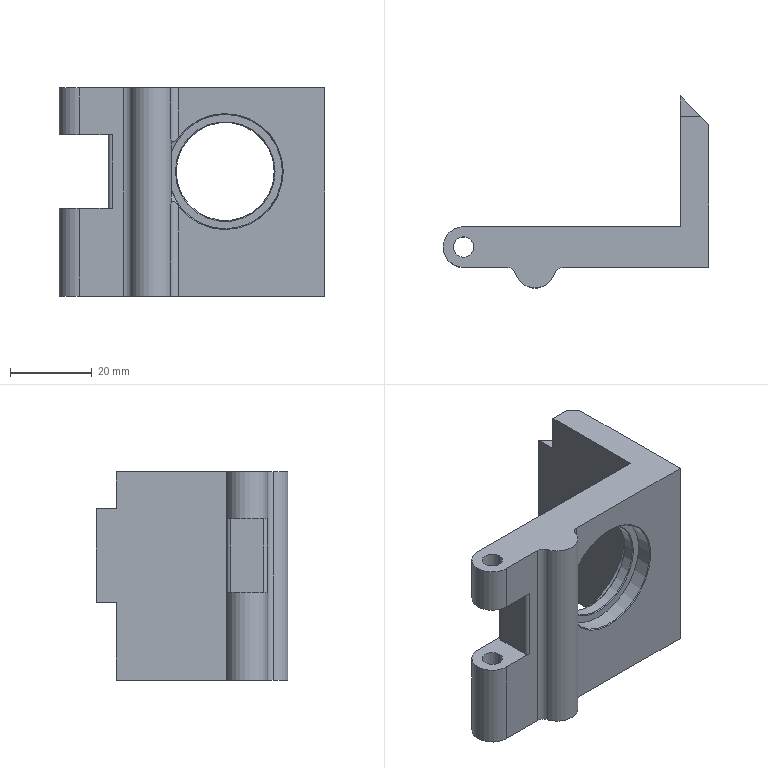Part | Creo | features CURVE 9, CUT 5, PROTRUSION 4, DATUM PLANE 3, ROUND 3, CHAMFER 2, COORDINATE SYSTEM 1 | 1 solid | 42 faces | box 65 x 47 x 51 mm | volume 35916 mm3 | cylinder 18 | plane 17 | cone 7 | commonest cylinder face diameters 5 x4 4 x3 10 x3 2 x2 24 x2 28 x2
STEP:
#1=CARTESIAN_POINT('',(0.,0.,0.));
#2=DIRECTION('',(0.,0.,1.));
#3=DIRECTION('',(1.,0.,0.));
#4=AXIS2_PLACEMENT_3D('',#1,#2,#3);
#5=CARTESIAN_POINT('',(28.,37.,20.5));
#6=VERTEX_POINT('',#5);
#7=CARTESIAN_POINT('',(33.,37.,20.5));
#8=VERTEX_POINT('',#7);
#9=CARTESIAN_POINT('',(28.,37.,20.5));
#10=DIRECTION('',(1.,0.,0.));
#11=VECTOR('',#10,5.);
#12=LINE('',#9,#11);
#13=EDGE_CURVE('',#6,#8,#12,.T.);
#14=ORIENTED_EDGE('',*,*,#13,.T.);
#15=CARTESIAN_POINT('',(35.,35.,20.5));
#16=VERTEX_POINT('',#15);
#17=CARTESIAN_POINT('',(35.,35.,20.5));
#18=DIRECTION('',(-0.7071,0.7071,0.));
#19=VECTOR('',#18,2.828);
#20=LINE('',#17,#19);
#21=EDGE_CURVE('',#16,#8,#20,.T.);
#22=ORIENTED_EDGE('',*,*,#21,.F.);
#23=CARTESIAN_POINT('',(35.,0.,20.5));
#24=VERTEX_POINT('',#23);
#25=CARTESIAN_POINT('',(35.,35.,20.5));
#26=DIRECTION('',(0.,-1.,0.));
#27=VECTOR('',#26,35.);
#28=LINE('',#25,#27);
#29=EDGE_CURVE('',#16,#24,#28,.T.);
#30=ORIENTED_EDGE('',*,*,#29,.T.);
#31=CARTESIAN_POINT('',(-0.7918,0.,20.5));
#32=VERTEX_POINT('',#31);
#33=CARTESIAN_POINT('',(35.,0.,20.5));
#34=DIRECTION('',(-1.,0.,0.));
#35=VECTOR('',#34,35.792);
#36=LINE('',#33,#35);
#37=EDGE_CURVE('',#24,#32,#36,.T.);
#38=ORIENTED_EDGE('',*,*,#37,.T.);
#39=CARTESIAN_POINT('',(-2.708,-1.429,20.5));
#40=VERTEX_POINT('',#39);
#41=CARTESIAN_POINT('',(-0.7918,-2.,20.5));
#42=DIRECTION('',(0.,0.,-1.));
#43=DIRECTION('',(-0.9583,0.2857,0.));
#44=AXIS2_PLACEMENT_3D('',#41,#42,#43);
#45=CIRCLE('',#44,2.);
#46=EDGE_CURVE('',#40,#32,#45,.T.);
#47=ORIENTED_EDGE('',*,*,#46,.F.);
#48=CARTESIAN_POINT('',(-12.292,-1.429,20.5));
#49=VERTEX_POINT('',#48);
#50=CARTESIAN_POINT('',(-7.5,0.,20.5));
#51=DIRECTION('',(0.,0.,1.));
#52=DIRECTION('',(-0.9583,-0.2857,0.));
#53=AXIS2_PLACEMENT_3D('',#50,#51,#52);
#54=CIRCLE('',#53,5.);
#55=EDGE_CURVE('',#49,#40,#54,.T.);
#56=ORIENTED_EDGE('',*,*,#55,.F.);
#57=CARTESIAN_POINT('',(-14.208,0.,20.5));
#58=VERTEX_POINT('',#57);
#59=CARTESIAN_POINT('',(-14.208,-2.,20.5));
#60=DIRECTION('',(0.,0.,-1.));
#61=DIRECTION('',(0.,1.,0.));
#62=AXIS2_PLACEMENT_3D('',#59,#60,#61);
#63=CIRCLE('',#62,2.);
#64=EDGE_CURVE('',#58,#49,#63,.T.);
#65=ORIENTED_EDGE('',*,*,#64,.F.);
#66=CARTESIAN_POINT('',(-25.,0.,20.5));
#67=VERTEX_POINT('',#66);
#68=CARTESIAN_POINT('',(-25.,0.,20.5));
#69=DIRECTION('',(1.,0.,0.));
#70=VECTOR('',#69,10.792);
#71=LINE('',#68,#70);
#72=EDGE_CURVE('',#67,#58,#71,.T.);
#73=ORIENTED_EDGE('',*,*,#72,.F.);
#74=CARTESIAN_POINT('',(-25.,10.,20.5));
#75=VERTEX_POINT('',#74);
#76=CARTESIAN_POINT('',(-25.,5.,20.5));
#77=DIRECTION('',(0.,0.,-1.));
#78=DIRECTION('',(0.,-1.,0.));
#79=AXIS2_PLACEMENT_3D('',#76,#77,#78);
#80=CIRCLE('',#79,5.);
#81=EDGE_CURVE('',#67,#75,#80,.T.);
#82=ORIENTED_EDGE('',*,*,#81,.T.);
#83=CARTESIAN_POINT('',(28.,10.,20.5));
#84=VERTEX_POINT('',#83);
#85=CARTESIAN_POINT('',(28.,10.,20.5));
#86=DIRECTION('',(-1.,0.,0.));
#87=VECTOR('',#86,53.);
#88=LINE('',#85,#87);
#89=EDGE_CURVE('',#84,#75,#88,.T.);
#90=ORIENTED_EDGE('',*,*,#89,.F.);
#91=CARTESIAN_POINT('',(28.,37.,20.5));
#92=DIRECTION('',(0.,-1.,0.));
#93=VECTOR('',#92,27.);
#94=LINE('',#91,#93);
#95=EDGE_CURVE('',#6,#84,#94,.T.);
#96=ORIENTED_EDGE('',*,*,#95,.F.);
#97=EDGE_LOOP('',(#14,#22,#30,#38,#47,#56,#65,#73,#82,#90,#96));
#98=FACE_OUTER_BOUND('',#97,.F.);
#99=CARTESIAN_POINT('',(-22.5,5.,20.5));
#100=VERTEX_POINT('',#99);
#101=CARTESIAN_POINT('',(-27.5,5.,20.5));
#102=VERTEX_POINT('',#101);
#103=CARTESIAN_POINT('',(-25.,5.,20.5));
#104=DIRECTION('',(0.,0.,-1.));
#105=DIRECTION('',(1.,0.,0.));
#106=AXIS2_PLACEMENT_3D('',#103,#104,#105);
#107=CIRCLE('',#106,2.5);
#108=EDGE_CURVE('',#100,#102,#107,.T.);
#109=ORIENTED_EDGE('',*,*,#108,.F.);
#110=CARTESIAN_POINT('',(-25.,5.,20.5));
#111=DIRECTION('',(0.,0.,-1.));
#112=DIRECTION('',(-1.,0.,0.));
#113=AXIS2_PLACEMENT_3D('',#110,#111,#112);
#114=CIRCLE('',#113,2.5);
#115=EDGE_CURVE('',#102,#100,#114,.T.);
#116=ORIENTED_EDGE('',*,*,#115,.F.);
#117=EDGE_LOOP('',(#109,#116));
#118=FACE_BOUND('',#117,.F.);
#119=CARTESIAN_POINT('',(0.,0.,20.5));
#120=DIRECTION('',(0.,0.,1.));
#121=DIRECTION('',(1.,0.,0.));
#122=AXIS2_PLACEMENT_3D('',#119,#120,#121);
#123=PLANE('',#122);
#124=ADVANCED_FACE('',(#98,#118),#123,.T.);
#125=CARTESIAN_POINT('',(-27.5,5.,9.));
#126=VERTEX_POINT('',#125);
#127=CARTESIAN_POINT('',(-22.5,5.,9.));
#128=VERTEX_POINT('',#127);
#129=CARTESIAN_POINT('',(-25.,5.,9.));
#130=DIRECTION('',(0.,0.,1.));
#131=DIRECTION('',(-1.,0.,0.));
#132=AXIS2_PLACEMENT_3D('',#129,#130,#131);
#133=CIRCLE('',#132,2.5);
#134=EDGE_CURVE('',#126,#128,#133,.T.);
#135=ORIENTED_EDGE('',*,*,#134,.T.);
#136=CARTESIAN_POINT('',(-22.5,5.,9.));
#137=DIRECTION('',(0.,0.,1.));
#138=VECTOR('',#137,11.5);
#139=LINE('',#136,#138);
#140=EDGE_CURVE('',#128,#100,#139,.T.);
#141=ORIENTED_EDGE('',*,*,#140,.T.);
#142=ORIENTED_EDGE('',*,*,#108,.T.);
#143=CARTESIAN_POINT('',(-27.5,5.,9.));
#144=DIRECTION('',(0.,0.,1.));
#145=VECTOR('',#144,11.5);
#146=LINE('',#143,#145);
#147=EDGE_CURVE('',#126,#102,#146,.T.);
#148=ORIENTED_EDGE('',*,*,#147,.F.);
#149=EDGE_LOOP('',(#135,#141,#142,#148));
#150=FACE_OUTER_BOUND('',#149,.F.);
#151=CARTESIAN_POINT('',(-25.,5.,-20.5));
#152=DIRECTION('',(0.,0.,1.));
#153=DIRECTION('',(1.,0.,0.));
#154=AXIS2_PLACEMENT_3D('',#151,#152,#153);
#155=CYLINDRICAL_SURFACE('',#154,2.5);
#156=ADVANCED_FACE('',(#150),#155,.F.);
#157=CARTESIAN_POINT('',(-27.5,5.,-9.));
#158=VERTEX_POINT('',#157);
#159=CARTESIAN_POINT('',(-27.5,5.,-30.5));
#160=VERTEX_POINT('',#159);
#161=CARTESIAN_POINT('',(-27.5,5.,-9.));
#162=DIRECTION('',(0.,0.,-1.));
#163=VECTOR('',#162,21.5);
#164=LINE('',#161,#163);
#165=EDGE_CURVE('',#158,#160,#164,.T.);
#166=ORIENTED_EDGE('',*,*,#165,.T.);
#167=CARTESIAN_POINT('',(-22.5,5.,-30.5));
#168=VERTEX_POINT('',#167);
#169=CARTESIAN_POINT('',(-25.,5.,-30.5));
#170=DIRECTION('',(0.,0.,1.));
#171=DIRECTION('',(-1.,0.,0.));
#172=AXIS2_PLACEMENT_3D('',#169,#170,#171);
#173=CIRCLE('',#172,2.5);
#174=EDGE_CURVE('',#160,#168,#173,.T.);
#175=ORIENTED_EDGE('',*,*,#174,.T.);
#176=CARTESIAN_POINT('',(-22.5,5.,-9.));
#177=VERTEX_POINT('',#176);
#178=CARTESIAN_POINT('',(-22.5,5.,-30.5));
#179=DIRECTION('',(0.,0.,1.));
#180=VECTOR('',#179,21.5);
#181=LINE('',#178,#180);
#182=EDGE_CURVE('',#168,#177,#181,.T.);
#183=ORIENTED_EDGE('',*,*,#182,.T.);
#184=CARTESIAN_POINT('',(-25.,5.,-9.));
#185=DIRECTION('',(0.,0.,1.));
#186=DIRECTION('',(-1.,0.,0.));
#187=AXIS2_PLACEMENT_3D('',#184,#185,#186);
#188=CIRCLE('',#187,2.5);
#189=EDGE_CURVE('',#158,#177,#188,.T.);
#190=ORIENTED_EDGE('',*,*,#189,.F.);
#191=EDGE_LOOP('',(#166,#175,#183,#190));
#192=FACE_OUTER_BOUND('',#191,.F.);
#193=CARTESIAN_POINT('',(-25.,5.,-20.5));
#194=DIRECTION('',(0.,0.,1.));
#195=DIRECTION('',(1.,0.,0.));
#196=AXIS2_PLACEMENT_3D('',#193,#194,#195);
#197=CYLINDRICAL_SURFACE('',#196,2.5);
#198=ADVANCED_FACE('',(#192),#197,.F.);
#199=CARTESIAN_POINT('',(-25.,0.,9.));
#200=VERTEX_POINT('',#199);
#201=CARTESIAN_POINT('',(-17.,0.,9.));
#202=VERTEX_POINT('',#201);
#203=CARTESIAN_POINT('',(-25.,0.,9.));
#204=DIRECTION('',(1.,0.,0.));
#205=VECTOR('',#204,8.);
#206=LINE('',#203,#205);
#207=EDGE_CURVE('',#200,#202,#206,.T.);
#208=ORIENTED_EDGE('',*,*,#207,.T.);
#209=CARTESIAN_POINT('',(-18.,1.,9.));
#210=VERTEX_POINT('',#209);
#211=CARTESIAN_POINT('',(-17.,1.,9.));
#212=DIRECTION('',(0.,0.,1.));
#213=DIRECTION('',(-1.,0.,0.));
#214=AXIS2_PLACEMENT_3D('',#211,#212,#213);
#215=CIRCLE('',#214,1.);
#216=EDGE_CURVE('',#210,#202,#215,.T.);
#217=ORIENTED_EDGE('',*,*,#216,.F.);
#218=CARTESIAN_POINT('',(-18.,9.,9.));
#219=VERTEX_POINT('',#218);
#220=CARTESIAN_POINT('',(-18.,9.,9.));
#221=DIRECTION('',(0.,-1.,0.));
#222=VECTOR('',#221,8.);
#223=LINE('',#220,#222);
#224=EDGE_CURVE('',#219,#210,#223,.T.);
#225=ORIENTED_EDGE('',*,*,#224,.F.);
#226=CARTESIAN_POINT('',(-17.,10.,9.));
#227=VERTEX_POINT('',#226);
#228=CARTESIAN_POINT('',(-17.,9.,9.));
#229=DIRECTION('',(0.,0.,1.));
#230=DIRECTION('',(0.,1.,0.));
#231=AXIS2_PLACEMENT_3D('',#228,#229,#230);
#232=CIRCLE('',#231,1.);
#233=EDGE_CURVE('',#227,#219,#232,.T.);
#234=ORIENTED_EDGE('',*,*,#233,.F.);
#235=CARTESIAN_POINT('',(-25.,10.,9.));
#236=VERTEX_POINT('',#235);
#237=CARTESIAN_POINT('',(-17.,10.,9.));
#238=DIRECTION('',(-1.,0.,0.));
#239=VECTOR('',#238,8.);
#240=LINE('',#237,#239);
#241=EDGE_CURVE('',#227,#236,#240,.T.);
#242=ORIENTED_EDGE('',*,*,#241,.T.);
#243=CARTESIAN_POINT('',(-25.,5.,9.));
#244=DIRECTION('',(0.,0.,1.));
#245=DIRECTION('',(0.,1.,0.));
#246=AXIS2_PLACEMENT_3D('',#243,#244,#245);
#247=CIRCLE('',#246,5.);
#248=EDGE_CURVE('',#236,#200,#247,.T.);
#249=ORIENTED_EDGE('',*,*,#248,.T.);
#250=EDGE_LOOP('',(#208,#217,#225,#234,#242,#249));
#251=FACE_OUTER_BOUND('',#250,.F.);
#252=ORIENTED_EDGE('',*,*,#134,.F.);
#253=CARTESIAN_POINT('',(-25.,5.,9.));
#254=DIRECTION('',(0.,0.,1.));
#255=DIRECTION('',(1.,0.,0.));
#256=AXIS2_PLACEMENT_3D('',#253,#254,#255);
#257=CIRCLE('',#256,2.5);
#258=EDGE_CURVE('',#128,#126,#257,.T.);
#259=ORIENTED_EDGE('',*,*,#258,.F.);
#260=EDGE_LOOP('',(#252,#259));
#261=FACE_BOUND('',#260,.F.);
#262=CARTESIAN_POINT('',(-30.,10.,9.));
#263=DIRECTION('',(0.,0.,1.));
#264=DIRECTION('',(1.,0.,0.));
#265=AXIS2_PLACEMENT_3D('',#262,#263,#264);
#266=PLANE('',#265);
#267=ADVANCED_FACE('',(#251,#261),#266,.F.);
#268=ORIENTED_EDGE('',*,*,#258,.T.);
#269=ORIENTED_EDGE('',*,*,#147,.T.);
#270=ORIENTED_EDGE('',*,*,#115,.T.);
#271=ORIENTED_EDGE('',*,*,#140,.F.);
#272=EDGE_LOOP('',(#268,#269,#270,#271));
#273=FACE_OUTER_BOUND('',#272,.F.);
#274=CARTESIAN_POINT('',(-25.,5.,-20.5));
#275=DIRECTION('',(0.,0.,1.));
#276=DIRECTION('',(1.,0.,0.));
#277=AXIS2_PLACEMENT_3D('',#274,#275,#276);
#278=CYLINDRICAL_SURFACE('',#277,2.5);
#279=ADVANCED_FACE('',(#273),#278,.F.);
#280=ORIENTED_EDGE('',*,*,#182,.F.);
#281=CARTESIAN_POINT('',(-25.,5.,-30.5));
#282=DIRECTION('',(0.,0.,1.));
#283=DIRECTION('',(1.,0.,0.));
#284=AXIS2_PLACEMENT_3D('',#281,#282,#283);
#285=CIRCLE('',#284,2.5);
#286=EDGE_CURVE('',#168,#160,#285,.T.);
#287=ORIENTED_EDGE('',*,*,#286,.T.);
#288=ORIENTED_EDGE('',*,*,#165,.F.);
#289=CARTESIAN_POINT('',(-25.,5.,-9.));
#290=DIRECTION('',(0.,0.,1.));
#291=DIRECTION('',(1.,0.,0.));
#292=AXIS2_PLACEMENT_3D('',#289,#290,#291);
#293=CIRCLE('',#292,2.5);
#294=EDGE_CURVE('',#177,#158,#293,.T.);
#295=ORIENTED_EDGE('',*,*,#294,.F.);
#296=EDGE_LOOP('',(#280,#287,#288,#295));
#297=FACE_OUTER_BOUND('',#296,.F.);
#298=CARTESIAN_POINT('',(-25.,5.,-20.5));
#299=DIRECTION('',(0.,0.,1.));
#300=DIRECTION('',(1.,0.,0.));
#301=AXIS2_PLACEMENT_3D('',#298,#299,#300);
#302=CYLINDRICAL_SURFACE('',#301,2.5);
#303=ADVANCED_FACE('',(#297),#302,.F.);
#304=CARTESIAN_POINT('',(33.,37.,-30.5));
#305=VERTEX_POINT('',#304);
#306=CARTESIAN_POINT('',(28.,37.,-30.5));
#307=VERTEX_POINT('',#306);
#308=CARTESIAN_POINT('',(33.,37.,-30.5));
#309=DIRECTION('',(-1.,0.,0.));
#310=VECTOR('',#309,5.);
#311=LINE('',#308,#310);
#312=EDGE_CURVE('',#305,#307,#311,.T.);
#313=ORIENTED_EDGE('',*,*,#312,.T.);
#314=CARTESIAN_POINT('',(28.,10.,-30.5));
#315=VERTEX_POINT('',#314);
#316=CARTESIAN_POINT('',(28.,10.,-30.5));
#317=DIRECTION('',(0.,1.,0.));
#318=VECTOR('',#317,27.);
#319=LINE('',#316,#318);
#320=EDGE_CURVE('',#315,#307,#319,.T.);
#321=ORIENTED_EDGE('',*,*,#320,.F.);
#322=CARTESIAN_POINT('',(-25.,10.,-30.5));
#323=VERTEX_POINT('',#322);
#324=CARTESIAN_POINT('',(-25.,10.,-30.5));
#325=DIRECTION('',(1.,0.,0.));
#326=VECTOR('',#325,53.);
#327=LINE('',#324,#326);
#328=EDGE_CURVE('',#323,#315,#327,.T.);
#329=ORIENTED_EDGE('',*,*,#328,.F.);
#330=CARTESIAN_POINT('',(-25.,0.,-30.5));
#331=VERTEX_POINT('',#330);
#332=CARTESIAN_POINT('',(-25.,5.,-30.5));
#333=DIRECTION('',(0.,0.,-1.));
#334=DIRECTION('',(0.,-1.,0.));
#335=AXIS2_PLACEMENT_3D('',#332,#333,#334);
#336=CIRCLE('',#335,5.);
#337=EDGE_CURVE('',#331,#323,#336,.T.);
#338=ORIENTED_EDGE('',*,*,#337,.F.);
#339=CARTESIAN_POINT('',(-14.208,0.,-30.5));
#340=VERTEX_POINT('',#339);
#341=CARTESIAN_POINT('',(-14.208,0.,-30.5));
#342=DIRECTION('',(-1.,0.,0.));
#343=VECTOR('',#342,10.792);
#344=LINE('',#341,#343);
#345=EDGE_CURVE('',#340,#331,#344,.T.);
#346=ORIENTED_EDGE('',*,*,#345,.F.);
#347=CARTESIAN_POINT('',(-12.292,-1.429,-30.5));
#348=VERTEX_POINT('',#347);
#349=CARTESIAN_POINT('',(-14.208,-2.,-30.5));
#350=DIRECTION('',(0.,0.,1.));
#351=DIRECTION('',(0.9583,0.2857,0.));
#352=AXIS2_PLACEMENT_3D('',#349,#350,#351);
#353=CIRCLE('',#352,2.);
#354=EDGE_CURVE('',#348,#340,#353,.T.);
#355=ORIENTED_EDGE('',*,*,#354,.F.);
#356=CARTESIAN_POINT('',(-2.708,-1.429,-30.5));
#357=VERTEX_POINT('',#356);
#358=CARTESIAN_POINT('',(-7.5,0.,-30.5));
#359=DIRECTION('',(0.,0.,-1.));
#360=DIRECTION('',(0.9583,-0.2857,0.));
#361=AXIS2_PLACEMENT_3D('',#358,#359,#360);
#362=CIRCLE('',#361,5.);
#363=EDGE_CURVE('',#357,#348,#362,.T.);
#364=ORIENTED_EDGE('',*,*,#363,.F.);
#365=CARTESIAN_POINT('',(-0.7918,0.,-30.5));
#366=VERTEX_POINT('',#365);
#367=CARTESIAN_POINT('',(-0.7918,-2.,-30.5));
#368=DIRECTION('',(0.,0.,1.));
#369=DIRECTION('',(0.,1.,0.));
#370=AXIS2_PLACEMENT_3D('',#367,#368,#369);
#371=CIRCLE('',#370,2.);
#372=EDGE_CURVE('',#366,#357,#371,.T.);
#373=ORIENTED_EDGE('',*,*,#372,.F.);
#374=CARTESIAN_POINT('',(35.,0.,-30.5));
#375=VERTEX_POINT('',#374);
#376=CARTESIAN_POINT('',(-0.7918,0.,-30.5));
#377=DIRECTION('',(1.,0.,0.));
#378=VECTOR('',#377,35.792);
#379=LINE('',#376,#378);
#380=EDGE_CURVE('',#366,#375,#379,.T.);
#381=ORIENTED_EDGE('',*,*,#380,.T.);
#382=CARTESIAN_POINT('',(35.,35.,-30.5));
#383=VERTEX_POINT('',#382);
#384=CARTESIAN_POINT('',(35.,0.,-30.5));
#385=DIRECTION('',(0.,1.,0.));
#386=VECTOR('',#385,35.);
#387=LINE('',#384,#386);
#388=EDGE_CURVE('',#375,#383,#387,.T.);
#389=ORIENTED_EDGE('',*,*,#388,.T.);
#390=CARTESIAN_POINT('',(33.,37.,-30.5));
#391=DIRECTION('',(0.7071,-0.7071,0.));
#392=VECTOR('',#391,2.828);
#393=LINE('',#390,#392);
#394=EDGE_CURVE('',#305,#383,#393,.T.);
#395=ORIENTED_EDGE('',*,*,#394,.F.);
#396=EDGE_LOOP('',(#313,#321,#329,#338,#346,#355,#364,#373,#381,#389,#395));
#397=FACE_OUTER_BOUND('',#396,.F.);
#398=ORIENTED_EDGE('',*,*,#286,.F.);
#399=ORIENTED_EDGE('',*,*,#174,.F.);
#400=EDGE_LOOP('',(#398,#399));
#401=FACE_BOUND('',#400,.F.);
#402=CARTESIAN_POINT('',(0.,0.,-30.5));
#403=DIRECTION('',(0.,0.,-1.));
#404=DIRECTION('',(-1.,0.,0.));
#405=AXIS2_PLACEMENT_3D('',#402,#403,#404);
#406=PLANE('',#405);
#407=ADVANCED_FACE('',(#397,#401),#406,.T.);
#408=CARTESIAN_POINT('',(28.,37.,-11.5));
#409=VERTEX_POINT('',#408);
#410=CARTESIAN_POINT('',(28.,37.,-30.5));
#411=DIRECTION('',(0.,0.,1.));
#412=VECTOR('',#411,19.);
#413=LINE('',#410,#412);
#414=EDGE_CURVE('',#307,#409,#413,.T.);
#415=ORIENTED_EDGE('',*,*,#414,.F.);
#416=ORIENTED_EDGE('',*,*,#312,.F.);
#417=CARTESIAN_POINT('',(33.,37.,-11.5));
#418=VERTEX_POINT('',#417);
#419=CARTESIAN_POINT('',(33.,37.,-30.5));
#420=DIRECTION('',(0.,0.,1.));
#421=VECTOR('',#420,19.);
#422=LINE('',#419,#421);
#423=EDGE_CURVE('',#305,#418,#422,.T.);
#424=ORIENTED_EDGE('',*,*,#423,.T.);
#425=CARTESIAN_POINT('',(33.,37.,-11.5));
#426=DIRECTION('',(-1.,0.,0.));
#427=VECTOR('',#426,5.);
#428=LINE('',#425,#427);
#429=EDGE_CURVE('',#418,#409,#428,.T.);
#430=ORIENTED_EDGE('',*,*,#429,.T.);
#431=EDGE_LOOP('',(#415,#416,#424,#430));
#432=FACE_OUTER_BOUND('',#431,.F.);
#433=CARTESIAN_POINT('',(35.,37.,-11.5));
#434=DIRECTION('',(0.,-1.,0.));
#435=DIRECTION('',(0.,0.,-1.));
#436=AXIS2_PLACEMENT_3D('',#433,#434,#435);
#437=PLANE('',#436);
#438=ADVANCED_FACE('',(#432),#437,.F.);
#439=CARTESIAN_POINT('',(28.,42.,-11.5));
#440=VERTEX_POINT('',#439);
#441=CARTESIAN_POINT('',(28.,42.,-11.5));
#442=DIRECTION('',(0.,-1.,0.));
#443=VECTOR('',#442,5.);
#444=LINE('',#441,#443);
#445=EDGE_CURVE('',#440,#409,#444,.T.);
#446=ORIENTED_EDGE('',*,*,#445,.F.);
#447=CARTESIAN_POINT('',(28.,42.,11.5));
#448=VERTEX_POINT('',#447);
#449=CARTESIAN_POINT('',(28.,42.,-11.5));
#450=DIRECTION('',(0.,0.,1.));
#451=VECTOR('',#450,23.);
#452=LINE('',#449,#451);
#453=EDGE_CURVE('',#440,#448,#452,.T.);
#454=ORIENTED_EDGE('',*,*,#453,.T.);
#455=CARTESIAN_POINT('',(28.,37.,11.5));
#456=VERTEX_POINT('',#455);
#457=CARTESIAN_POINT('',(28.,42.,11.5));
#458=DIRECTION('',(0.,-1.,0.));
#459=VECTOR('',#458,5.);
#460=LINE('',#457,#459);
#461=EDGE_CURVE('',#448,#456,#460,.T.);
#462=ORIENTED_EDGE('',*,*,#461,.T.);
#463=CARTESIAN_POINT('',(28.,37.,20.5));
#464=DIRECTION('',(0.,0.,-1.));
#465=VECTOR('',#464,9.);
#466=LINE('',#463,#465);
#467=EDGE_CURVE('',#6,#456,#466,.T.);
#468=ORIENTED_EDGE('',*,*,#467,.F.);
#469=ORIENTED_EDGE('',*,*,#95,.T.);
#470=CARTESIAN_POINT('',(28.,10.,20.5));
#471=DIRECTION('',(0.,0.,-1.));
#472=VECTOR('',#471,51.);
#473=LINE('',#470,#472);
#474=EDGE_CURVE('',#84,#315,#473,.T.);
#475=ORIENTED_EDGE('',*,*,#474,.T.);
#476=ORIENTED_EDGE('',*,*,#320,.T.);
#477=ORIENTED_EDGE('',*,*,#414,.T.);
#478=EDGE_LOOP('',(#446,#454,#462,#468,#469,#475,#476,#477));
#479=FACE_OUTER_BOUND('',#478,.F.);
#480=CARTESIAN_POINT('',(28.,42.,-20.5));
#481=DIRECTION('',(-1.,0.,0.));
#482=DIRECTION('',(0.,-1.,0.));
#483=AXIS2_PLACEMENT_3D('',#480,#481,#482);
#484=PLANE('',#483);
#485=ADVANCED_FACE('',(#479),#484,.T.);
#486=ORIENTED_EDGE('',*,*,#445,.T.);
#487=ORIENTED_EDGE('',*,*,#429,.F.);
#488=CARTESIAN_POINT('',(28.,42.,-11.5));
#489=DIRECTION('',(0.7071,-0.7071,0.));
#490=VECTOR('',#489,7.071);
#491=LINE('',#488,#490);
#492=EDGE_CURVE('',#440,#418,#491,.T.);
#493=ORIENTED_EDGE('',*,*,#492,.F.);
#494=EDGE_LOOP('',(#486,#487,#493));
#495=FACE_OUTER_BOUND('',#494,.F.);
#496=CARTESIAN_POINT('',(35.,42.,-11.5));
#497=DIRECTION('',(0.,0.,1.));
#498=DIRECTION('',(0.,-1.,0.));
#499=AXIS2_PLACEMENT_3D('',#496,#497,#498);
#500=PLANE('',#499);
#501=ADVANCED_FACE('',(#495),#500,.F.);
#502=ORIENTED_EDGE('',*,*,#492,.T.);
#503=ORIENTED_EDGE('',*,*,#423,.F.);
#504=ORIENTED_EDGE('',*,*,#394,.T.);
#505=CARTESIAN_POINT('',(35.,35.,-30.5));
#506=DIRECTION('',(0.,0.,1.));
#507=VECTOR('',#506,51.);
#508=LINE('',#505,#507);
#509=EDGE_CURVE('',#383,#16,#508,.T.);
#510=ORIENTED_EDGE('',*,*,#509,.T.);
#511=ORIENTED_EDGE('',*,*,#21,.T.);
#512=CARTESIAN_POINT('',(33.,37.,11.5));
#513=VERTEX_POINT('',#512);
#514=CARTESIAN_POINT('',(33.,37.,20.5));
#515=DIRECTION('',(0.,0.,-1.));
#516=VECTOR('',#515,9.);
#517=LINE('',#514,#516);
#518=EDGE_CURVE('',#8,#513,#517,.T.);
#519=ORIENTED_EDGE('',*,*,#518,.T.);
#520=CARTESIAN_POINT('',(28.,42.,11.5));
#521=DIRECTION('',(0.7071,-0.7071,0.));
#522=VECTOR('',#521,7.071);
#523=LINE('',#520,#522);
#524=EDGE_CURVE('',#448,#513,#523,.T.);
#525=ORIENTED_EDGE('',*,*,#524,.F.);
#526=ORIENTED_EDGE('',*,*,#453,.F.);
#527=EDGE_LOOP('',(#502,#503,#504,#510,#511,#519,#525,#526));
#528=FACE_OUTER_BOUND('',#527,.F.);
#529=CARTESIAN_POINT('',(31.5,38.5,-5.));
#530=DIRECTION('',(0.7071,0.7071,0.));
#531=DIRECTION('',(-0.7071,0.7071,0.));
#532=AXIS2_PLACEMENT_3D('',#529,#530,#531);
#533=PLANE('',#532);
#534=ADVANCED_FACE('',(#528),#533,.T.);
#535=ORIENTED_EDGE('',*,*,#509,.F.);
#536=ORIENTED_EDGE('',*,*,#388,.F.);
#537=CARTESIAN_POINT('',(35.,0.,20.5));
#538=DIRECTION('',(0.,0.,-1.));
#539=VECTOR('',#538,51.);
#540=LINE('',#537,#539);
#541=EDGE_CURVE('',#24,#375,#540,.T.);
#542=ORIENTED_EDGE('',*,*,#541,.F.);
#543=ORIENTED_EDGE('',*,*,#29,.F.);
#544=EDGE_LOOP('',(#535,#536,#542,#543));
#545=FACE_OUTER_BOUND('',#544,.F.);
#546=CARTESIAN_POINT('',(35.,0.,20.5));
#547=DIRECTION('',(1.,0.,0.));
#548=DIRECTION('',(0.,0.,-1.));
#549=AXIS2_PLACEMENT_3D('',#546,#547,#548);
#550=PLANE('',#549);
#551=ADVANCED_FACE('',(#545),#550,.T.);
#552=CARTESIAN_POINT('',(-14.208,0.,-30.5));
#553=DIRECTION('',(0.,0.,1.));
#554=VECTOR('',#553,51.);
#555=LINE('',#552,#554);
#556=EDGE_CURVE('',#340,#58,#555,.T.);
#557=ORIENTED_EDGE('',*,*,#556,.F.);
#558=ORIENTED_EDGE('',*,*,#345,.T.);
#559=CARTESIAN_POINT('',(-25.,0.,-9.));
#560=VERTEX_POINT('',#559);
#561=CARTESIAN_POINT('',(-25.,0.,-30.5));
#562=DIRECTION('',(0.,0.,1.));
#563=VECTOR('',#562,21.5);
#564=LINE('',#561,#563);
#565=EDGE_CURVE('',#331,#560,#564,.T.);
#566=ORIENTED_EDGE('',*,*,#565,.T.);
#567=CARTESIAN_POINT('',(-17.,0.,-9.));
#568=VERTEX_POINT('',#567);
#569=CARTESIAN_POINT('',(-17.,0.,-9.));
#570=DIRECTION('',(-1.,0.,0.));
#571=VECTOR('',#570,8.);
#572=LINE('',#569,#571);
#573=EDGE_CURVE('',#568,#560,#572,.T.);
#574=ORIENTED_EDGE('',*,*,#573,.F.);
#575=CARTESIAN_POINT('',(-17.,0.,9.));
#576=DIRECTION('',(0.,0.,-1.));
#577=VECTOR('',#576,18.);
#578=LINE('',#575,#577);
#579=EDGE_CURVE('',#202,#568,#578,.T.);
#580=ORIENTED_EDGE('',*,*,#579,.F.);
#581=ORIENTED_EDGE('',*,*,#207,.F.);
#582=CARTESIAN_POINT('',(-25.,0.,20.5));
#583=DIRECTION('',(0.,0.,-1.));
#584=VECTOR('',#583,11.5);
#585=LINE('',#582,#584);
#586=EDGE_CURVE('',#67,#200,#585,.T.);
#587=ORIENTED_EDGE('',*,*,#586,.F.);
#588=ORIENTED_EDGE('',*,*,#72,.T.);
#589=EDGE_LOOP('',(#557,#558,#566,#574,#580,#581,#587,#588));
#590=FACE_OUTER_BOUND('',#589,.F.);
#591=CARTESIAN_POINT('',(-30.,0.,-20.5));
#592=DIRECTION('',(0.,-1.,0.));
#593=DIRECTION('',(1.,0.,0.));
#594=AXIS2_PLACEMENT_3D('',#591,#592,#593);
#595=PLANE('',#594);
#596=ADVANCED_FACE('',(#590),#595,.T.);
#597=ORIENTED_EDGE('',*,*,#37,.F.);
#598=ORIENTED_EDGE('',*,*,#541,.T.);
#599=ORIENTED_EDGE('',*,*,#380,.F.);
#600=CARTESIAN_POINT('',(-0.7918,0.,-8.41));
#601=VERTEX_POINT('',#600);
#602=CARTESIAN_POINT('',(-0.7918,0.,-8.41));
#603=DIRECTION('',(0.,0.,-1.));
#604=VECTOR('',#603,22.09);
#605=LINE('',#602,#604);
#606=EDGE_CURVE('',#601,#366,#605,.T.);
#607=ORIENTED_EDGE('',*,*,#606,.F.);
#608=CARTESIAN_POINT('',(-0.7918,0.,8.41));
#609=VERTEX_POINT('',#608);
#610=CARTESIAN_POINT('',(10.65,0.,0.));
#611=DIRECTION('',(0.,1.,0.));
#612=DIRECTION('',(-0.8058,0.,0.5922));
#613=AXIS2_PLACEMENT_3D('',#610,#611,#612);
#614=CIRCLE('',#613,14.2);
#615=EDGE_CURVE('',#609,#601,#614,.T.);
#616=ORIENTED_EDGE('',*,*,#615,.F.);
#617=CARTESIAN_POINT('',(-0.7918,0.,8.41));
#618=DIRECTION('',(0.,0.,1.));
#619=VECTOR('',#618,12.09);
#620=LINE('',#617,#619);
#621=EDGE_CURVE('',#609,#32,#620,.T.);
#622=ORIENTED_EDGE('',*,*,#621,.T.);
#623=EDGE_LOOP('',(#597,#598,#599,#607,#616,#622));
#624=FACE_OUTER_BOUND('',#623,.F.);
#625=CARTESIAN_POINT('',(-30.,0.,-20.5));
#626=DIRECTION('',(0.,-1.,0.));
#627=DIRECTION('',(1.,0.,0.));
#628=AXIS2_PLACEMENT_3D('',#625,#626,#627);
#629=PLANE('',#628);
#630=ADVANCED_FACE('',(#624),#629,.T.);
#631=CARTESIAN_POINT('',(-12.292,-1.429,20.5));
#632=DIRECTION('',(0.,0.,-1.));
#633=VECTOR('',#632,51.);
#634=LINE('',#631,#633);
#635=EDGE_CURVE('',#49,#348,#634,.T.);
#636=ORIENTED_EDGE('',*,*,#635,.T.);
#637=ORIENTED_EDGE('',*,*,#354,.T.);
#638=ORIENTED_EDGE('',*,*,#556,.T.);
#639=ORIENTED_EDGE('',*,*,#64,.T.);
#640=EDGE_LOOP('',(#636,#637,#638,#639));
#641=FACE_OUTER_BOUND('',#640,.F.);
#642=CARTESIAN_POINT('',(-14.208,-2.,73.948));
#643=DIRECTION('',(0.,0.,-1.));
#644=DIRECTION('',(0.,1.,0.));
#645=AXIS2_PLACEMENT_3D('',#642,#643,#644);
#646=CYLINDRICAL_SURFACE('',#645,2.);
#647=ADVANCED_FACE('',(#641),#646,.F.);
#648=CARTESIAN_POINT('',(-2.708,-1.429,-8.112));
#649=VERTEX_POINT('',#648);
#650=CARTESIAN_POINT('',(-2.708,-1.429,-8.112));
#651=DIRECTION('',(0.,0.,-1.));
#652=VECTOR('',#651,22.388);
#653=LINE('',#650,#652);
#654=EDGE_CURVE('',#649,#357,#653,.T.);
#655=ORIENTED_EDGE('',*,*,#654,.T.);
#656=ORIENTED_EDGE('',*,*,#363,.T.);
#657=ORIENTED_EDGE('',*,*,#635,.F.);
#658=ORIENTED_EDGE('',*,*,#55,.T.);
#659=CARTESIAN_POINT('',(-2.708,-1.429,8.112));
#660=VERTEX_POINT('',#659);
#661=CARTESIAN_POINT('',(-2.708,-1.429,8.112));
#662=DIRECTION('',(0.,0.,1.));
#663=VECTOR('',#662,12.388);
#664=LINE('',#661,#663);
#665=EDGE_CURVE('',#660,#40,#664,.T.);
#666=ORIENTED_EDGE('',*,*,#665,.F.);
#667=CARTESIAN_POINT('',(-2.504,0.2,4.793));
#668=VERTEX_POINT('',#667);
#669=CARTESIAN_POINT('',(-2.504,0.2,4.793));
#670=CARTESIAN_POINT('',(-2.498,0.04859,5.252));
#671=CARTESIAN_POINT('',(-2.499,-0.2845,6.107));
#672=CARTESIAN_POINT('',(-2.56,-0.8402,7.207));
#673=CARTESIAN_POINT('',(-2.65,-1.231,7.829));
#674=CARTESIAN_POINT('',(-2.708,-1.429,8.112));
#675=B_SPLINE_CURVE_WITH_KNOTS('',3,(#669,#670,#671,#672,#673,#674),.UNSPECIFIED.,.F.,.F.,(4,1,1,4),(0.,0.3333,0.6667,1.),.UNSPECIFIED.);
#676=EDGE_CURVE('',#668,#660,#675,.T.);
#677=ORIENTED_EDGE('',*,*,#676,.F.);
#678=CARTESIAN_POINT('',(-3.35,2.789,0.));
#679=VERTEX_POINT('',#678);
#680=CARTESIAN_POINT('',(-3.35,2.789,0.1916));
#681=CARTESIAN_POINT('',(-3.342,2.777,0.5805));
#682=CARTESIAN_POINT('',(-3.303,2.719,1.196));
#683=CARTESIAN_POINT('',(-3.239,2.617,1.795));
#684=CARTESIAN_POINT('',(-3.155,2.476,2.348));
#685=CARTESIAN_POINT('',(-3.063,2.309,2.831));
#686=CARTESIAN_POINT('',(-2.97,2.121,3.245));
#687=CARTESIAN_POINT('',(-2.882,1.921,3.595));
#688=CARTESIAN_POINT('',(-2.798,1.706,3.896));
#689=CARTESIAN_POINT('',(-2.72,1.473,4.156));
#690=CARTESIAN_POINT('',(-2.644,1.205,4.39));
#691=CARTESIAN_POINT('',(-2.578,0.8999,4.586));
#692=CARTESIAN_POINT('',(-2.527,0.5585,4.729));
#693=CARTESIAN_POINT('',(-2.509,0.3219,4.78));
#694=B_SPLINE_CURVE_WITH_KNOTS('',3,(#678,#680,#681,#682,#683,#684,#685,#686,#687,#688,#689,#690,#691,#692,#693,#667),.UNSPECIFIED.,.F.,.F.,(4,1,1,1,1,1,1,1,1,1,1,1,1,4),(0.,0.07692,0.1538,0.2308,0.3077,0.3846,0.4615,0.5385,0.6154,0.6923,0.7692,0.8462,0.9231,1.),.UNSPECIFIED.);
#695=EDGE_CURVE('',#679,#668,#694,.T.);
#696=ORIENTED_EDGE('',*,*,#695,.F.);
#697=CARTESIAN_POINT('',(-2.504,0.2,-4.793));
#698=VERTEX_POINT('',#697);
#699=CARTESIAN_POINT('',(-2.51,0.3502,-4.776));
#700=CARTESIAN_POINT('',(-2.535,0.6438,-4.708));
#701=CARTESIAN_POINT('',(-2.611,1.077,-4.49));
#702=CARTESIAN_POINT('',(-2.714,1.463,-4.178));
#703=CARTESIAN_POINT('',(-2.836,1.815,-3.767));
#704=CARTESIAN_POINT('',(-2.968,2.119,-3.264));
#705=CARTESIAN_POINT('',(-3.094,2.368,-2.69));
#706=CARTESIAN_POINT('',(-3.204,2.561,-2.054));
#707=CARTESIAN_POINT('',(-3.289,2.696,-1.37));
#708=CARTESIAN_POINT('',(-3.34,2.773,-0.6702));
#709=CARTESIAN_POINT('',(-3.35,2.789,-0.2217));
#710=CARTESIAN_POINT('',(-3.35,2.789,0.));
#711=B_SPLINE_CURVE_WITH_KNOTS('',3,(#697,#699,#700,#701,#702,#703,#704,#705,#706,#707,#708,#709,#710),.UNSPECIFIED.,.F.,.F.,(4,1,1,1,1,1,1,1,1,1,4),(0.,0.1,0.2,0.3,0.4,0.5,0.6,0.7,0.8,0.9,1.),.UNSPECIFIED.);
#712=EDGE_CURVE('',#698,#679,#711,.T.);
#713=ORIENTED_EDGE('',*,*,#712,.F.);
#714=CARTESIAN_POINT('',(-2.708,-1.429,-8.112));
#715=CARTESIAN_POINT('',(-2.649,-1.229,-7.826));
#716=CARTESIAN_POINT('',(-2.559,-0.8359,-7.2));
#717=CARTESIAN_POINT('',(-2.499,-0.2807,-6.098));
#718=CARTESIAN_POINT('',(-2.498,0.04991,-5.248));
#719=CARTESIAN_POINT('',(-2.504,0.2,-4.793));
#720=B_SPLINE_CURVE_WITH_KNOTS('',3,(#714,#715,#716,#717,#718,#719),.UNSPECIFIED.,.F.,.F.,(4,1,1,4),(0.,0.3333,0.6667,1.),.UNSPECIFIED.);
#721=EDGE_CURVE('',#649,#698,#720,.T.);
#722=ORIENTED_EDGE('',*,*,#721,.F.);
#723=EDGE_LOOP('',(#655,#656,#657,#658,#666,#677,#696,#713,#722));
#724=FACE_OUTER_BOUND('',#723,.F.);
#725=CARTESIAN_POINT('',(-7.5,0.,20.5));
#726=DIRECTION('',(0.,0.,1.));
#727=DIRECTION('',(1.,0.,0.));
#728=AXIS2_PLACEMENT_3D('',#725,#726,#727);
#729=CYLINDRICAL_SURFACE('',#728,5.);
#730=ADVANCED_FACE('',(#724),#729,.T.);
#731=ORIENTED_EDGE('',*,*,#606,.T.);
#732=ORIENTED_EDGE('',*,*,#372,.T.);
#733=ORIENTED_EDGE('',*,*,#654,.F.);
#734=CARTESIAN_POINT('',(-2.685,-1.348,-7.997));
#735=CARTESIAN_POINT('',(-2.627,-1.191,-7.787));
#736=CARTESIAN_POINT('',(-2.509,-0.9632,-7.535));
#737=CARTESIAN_POINT('',(-2.353,-0.7397,-7.355));
#738=CARTESIAN_POINT('',(-2.154,-0.5259,-7.275));
#739=CARTESIAN_POINT('',(-1.941,-0.3562,-7.305));
#740=CARTESIAN_POINT('',(-1.728,-0.2271,-7.412));
#741=CARTESIAN_POINT('',(-1.509,-0.1279,-7.581));
#742=CARTESIAN_POINT('',(-1.282,-0.05592,-7.804));
#743=CARTESIAN_POINT('',(-1.042,-0.01059,-8.081));
#744=CARTESIAN_POINT('',(-0.8761,0.,-8.295));
#745=B_SPLINE_CURVE_WITH_KNOTS('',3,(#648,#734,#735,#736,#737,#738,#739,#740,#741,#742,#743,#744,#600),.UNSPECIFIED.,.F.,.F.,(4,1,1,1,1,1,1,1,1,1,4),(0.,0.1,0.2,0.3,0.4,0.5,0.6,0.7,0.8,0.9,1.),.UNSPECIFIED.);
#746=EDGE_CURVE('',#649,#601,#745,.T.);
#747=ORIENTED_EDGE('',*,*,#746,.T.);
#748=EDGE_LOOP('',(#731,#732,#733,#747));
#749=FACE_OUTER_BOUND('',#748,.F.);
#750=CARTESIAN_POINT('',(-0.7918,-2.,-73.948));
#751=DIRECTION('',(0.,0.,1.));
#752=DIRECTION('',(0.,1.,0.));
#753=AXIS2_PLACEMENT_3D('',#750,#751,#752);
#754=CYLINDRICAL_SURFACE('',#753,2.);
#755=ADVANCED_FACE('',(#749),#754,.F.);
#756=ORIENTED_EDGE('',*,*,#615,.T.);
#757=ORIENTED_EDGE('',*,*,#746,.F.);
#758=ORIENTED_EDGE('',*,*,#721,.T.);
#759=CARTESIAN_POINT('',(24.65,0.2,0.000000004));
#760=VERTEX_POINT('',#759);
#761=CARTESIAN_POINT('',(10.65,0.2,0.));
#762=DIRECTION('',(0.,1.,0.));
#763=DIRECTION('',(1.,0.,0.));
#764=AXIS2_PLACEMENT_3D('',#761,#762,#763);
#765=CIRCLE('',#764,14.);
#766=EDGE_CURVE('',#760,#698,#765,.T.);
#767=ORIENTED_EDGE('',*,*,#766,.F.);
#768=CARTESIAN_POINT('',(10.65,0.2,0.));
#769=DIRECTION('',(0.,1.,0.));
#770=DIRECTION('',(-0.9396,0.,0.3424));
#771=AXIS2_PLACEMENT_3D('',#768,#769,#770);
#772=CIRCLE('',#771,14.);
#773=EDGE_CURVE('',#668,#760,#772,.T.);
#774=ORIENTED_EDGE('',*,*,#773,.F.);
#775=ORIENTED_EDGE('',*,*,#676,.T.);
#776=CARTESIAN_POINT('',(-0.876,0.,8.295));
#777=CARTESIAN_POINT('',(-1.041,-0.01056,8.081));
#778=CARTESIAN_POINT('',(-1.281,-0.05579,7.805));
#779=CARTESIAN_POINT('',(-1.508,-0.1276,7.582));
#780=CARTESIAN_POINT('',(-1.727,-0.2265,7.413));
#781=CARTESIAN_POINT('',(-1.939,-0.3552,7.306));
#782=CARTESIAN_POINT('',(-2.153,-0.5252,7.275));
#783=CARTESIAN_POINT('',(-2.351,-0.7371,7.354));
#784=CARTESIAN_POINT('',(-2.507,-0.9596,7.531));
#785=CARTESIAN_POINT('',(-2.627,-1.19,7.785));
#786=CARTESIAN_POINT('',(-2.684,-1.348,7.996));
#787=B_SPLINE_CURVE_WITH_KNOTS('',3,(#608,#776,#777,#778,#779,#780,#781,#782,#783,#784,#785,#786,#659),.UNSPECIFIED.,.F.,.F.,(4,1,1,1,1,1,1,1,1,1,4),(0.,0.1,0.2,0.3,0.4,0.5,0.6,0.7,0.8,0.9,1.),.UNSPECIFIED.);
#788=EDGE_CURVE('',#609,#660,#787,.T.);
#789=ORIENTED_EDGE('',*,*,#788,.F.);
#790=EDGE_LOOP('',(#756,#757,#758,#767,#774,#775,#789));
#791=FACE_OUTER_BOUND('',#790,.F.);
#792=CARTESIAN_POINT('',(10.65,-0.6143,0.));
#793=DIRECTION('',(0.,-1.,0.));
#794=DIRECTION('',(0.,0.,-1.));
#795=AXIS2_PLACEMENT_3D('',#792,#793,#794);
#796=CONICAL_SURFACE('',#795,14.814,45.);
#797=ADVANCED_FACE('',(#791),#796,.F.);
#798=ORIENTED_EDGE('',*,*,#712,.T.);
#799=CARTESIAN_POINT('',(-3.35,4.,0.));
#800=VERTEX_POINT('',#799);
#801=CARTESIAN_POINT('',(-3.35,2.789,0.));
#802=DIRECTION('',(0.,1.,0.));
#803=VECTOR('',#802,1.211);
#804=LINE('',#801,#803);
#805=EDGE_CURVE('',#679,#800,#804,.T.);
#806=ORIENTED_EDGE('',*,*,#805,.T.);
#807=CARTESIAN_POINT('',(24.65,4.,0.));
#808=VERTEX_POINT('',#807);
#809=CARTESIAN_POINT('',(10.65,4.,0.));
#810=DIRECTION('',(0.,-1.,0.));
#811=DIRECTION('',(-1.,0.,0.));
#812=AXIS2_PLACEMENT_3D('',#809,#810,#811);
#813=CIRCLE('',#812,14.);
#814=EDGE_CURVE('',#800,#808,#813,.T.);
#815=ORIENTED_EDGE('',*,*,#814,.T.);
#816=CARTESIAN_POINT('',(24.65,0.2,0.000000004));
#817=DIRECTION('',(0.,1.,-0.000000001));
#818=VECTOR('',#817,3.8);
#819=LINE('',#816,#818);
#820=EDGE_CURVE('',#760,#808,#819,.T.);
#821=ORIENTED_EDGE('',*,*,#820,.F.);
#822=ORIENTED_EDGE('',*,*,#766,.T.);
#823=EDGE_LOOP('',(#798,#806,#815,#821,#822));
#824=FACE_OUTER_BOUND('',#823,.F.);
#825=CARTESIAN_POINT('',(10.65,0.,0.));
#826=DIRECTION('',(0.,-1.,0.));
#827=DIRECTION('',(1.,0.,0.));
#828=AXIS2_PLACEMENT_3D('',#825,#826,#827);
#829=CYLINDRICAL_SURFACE('',#828,14.);
#830=ADVANCED_FACE('',(#824),#829,.F.);
#831=ORIENTED_EDGE('',*,*,#695,.T.);
#832=ORIENTED_EDGE('',*,*,#773,.T.);
#833=ORIENTED_EDGE('',*,*,#820,.T.);
#834=CARTESIAN_POINT('',(10.65,4.,0.));
#835=DIRECTION('',(0.,-1.,0.));
#836=DIRECTION('',(1.,0.,0.));
#837=AXIS2_PLACEMENT_3D('',#834,#835,#836);
#838=CIRCLE('',#837,14.);
#839=EDGE_CURVE('',#808,#800,#838,.T.);
#840=ORIENTED_EDGE('',*,*,#839,.T.);
#841=ORIENTED_EDGE('',*,*,#805,.F.);
#842=EDGE_LOOP('',(#831,#832,#833,#840,#841));
#843=FACE_OUTER_BOUND('',#842,.F.);
#844=CARTESIAN_POINT('',(10.65,0.,0.));
#845=DIRECTION('',(0.,-1.,0.));
#846=DIRECTION('',(1.,0.,0.));
#847=AXIS2_PLACEMENT_3D('',#844,#845,#846);
#848=CYLINDRICAL_SURFACE('',#847,14.);
#849=ADVANCED_FACE('',(#843),#848,.F.);
#850=ORIENTED_EDGE('',*,*,#839,.F.);
#851=ORIENTED_EDGE('',*,*,#814,.F.);
#852=EDGE_LOOP('',(#850,#851));
#853=FACE_OUTER_BOUND('',#852,.F.);
#854=CARTESIAN_POINT('',(-1.55,4.,0.));
#855=VERTEX_POINT('',#854);
#856=CARTESIAN_POINT('',(22.85,4.,0.));
#857=VERTEX_POINT('',#856);
#858=CARTESIAN_POINT('',(10.65,4.,0.));
#859=DIRECTION('',(0.,-1.,0.));
#860=DIRECTION('',(-1.,0.,0.));
#861=AXIS2_PLACEMENT_3D('',#858,#859,#860);
#862=CIRCLE('',#861,12.2);
#863=EDGE_CURVE('',#855,#857,#862,.T.);
#864=ORIENTED_EDGE('',*,*,#863,.T.);
#865=CARTESIAN_POINT('',(10.65,4.,0.));
#866=DIRECTION('',(0.,-1.,0.));
#867=DIRECTION('',(1.,0.,0.));
#868=AXIS2_PLACEMENT_3D('',#865,#866,#867);
#869=CIRCLE('',#868,12.2);
#870=EDGE_CURVE('',#857,#855,#869,.T.);
#871=ORIENTED_EDGE('',*,*,#870,.T.);
#872=EDGE_LOOP('',(#864,#871));
#873=FACE_BOUND('',#872,.F.);
#874=CARTESIAN_POINT('',(0.,4.,-20.5));
#875=DIRECTION('',(0.,-1.,0.));
#876=DIRECTION('',(1.,0.,0.));
#877=AXIS2_PLACEMENT_3D('',#874,#875,#876);
#878=PLANE('',#877);
#879=ADVANCED_FACE('',(#853,#873),#878,.T.);
#880=CARTESIAN_POINT('',(-1.35,4.2,0.));
#881=VERTEX_POINT('',#880);
#882=CARTESIAN_POINT('',(22.65,4.2,0.));
#883=VERTEX_POINT('',#882);
#884=CARTESIAN_POINT('',(10.65,4.2,0.));
#885=DIRECTION('',(0.,-1.,0.));
#886=DIRECTION('',(-1.,0.,0.));
#887=AXIS2_PLACEMENT_3D('',#884,#885,#886);
#888=CIRCLE('',#887,12.);
#889=EDGE_CURVE('',#881,#883,#888,.T.);
#890=ORIENTED_EDGE('',*,*,#889,.T.);
#891=CARTESIAN_POINT('',(22.65,4.2,0.000000002));
#892=DIRECTION('',(0.7071,-0.7071,0.000000002));
#893=VECTOR('',#892,0.2828);
#894=LINE('',#891,#893);
#895=EDGE_CURVE('',#883,#857,#894,.T.);
#896=ORIENTED_EDGE('',*,*,#895,.T.);
#897=ORIENTED_EDGE('',*,*,#863,.F.);
#898=CARTESIAN_POINT('',(-1.35,4.2,-0.000000002));
#899=DIRECTION('',(-0.7071,-0.7071,-0.000000002));
#900=VECTOR('',#899,0.2828);
#901=LINE('',#898,#900);
#902=EDGE_CURVE('',#881,#855,#901,.T.);
#903=ORIENTED_EDGE('',*,*,#902,.F.);
#904=EDGE_LOOP('',(#890,#896,#897,#903));
#905=FACE_OUTER_BOUND('',#904,.F.);
#906=CARTESIAN_POINT('',(10.65,4.1,0.));
#907=DIRECTION('',(0.,-1.,0.));
#908=DIRECTION('',(0.,0.,-1.));
#909=AXIS2_PLACEMENT_3D('',#906,#907,#908);
#910=CONICAL_SURFACE('',#909,12.1,45.);
#911=ADVANCED_FACE('',(#905),#910,.F.);
#912=ORIENTED_EDGE('',*,*,#889,.F.);
#913=CARTESIAN_POINT('',(-1.35,6.8,0.));
#914=VERTEX_POINT('',#913);
#915=CARTESIAN_POINT('',(-1.35,6.8,0.000000006));
#916=DIRECTION('',(0.,-1.,-0.000000003));
#917=VECTOR('',#916,2.6);
#918=LINE('',#915,#917);
#919=EDGE_CURVE('',#914,#881,#918,.T.);
#920=ORIENTED_EDGE('',*,*,#919,.F.);
#921=CARTESIAN_POINT('',(22.65,6.8,0.));
#922=VERTEX_POINT('',#921);
#923=CARTESIAN_POINT('',(10.65,6.8,0.));
#924=DIRECTION('',(0.,-1.,0.));
#925=DIRECTION('',(-1.,0.,0.));
#926=AXIS2_PLACEMENT_3D('',#923,#924,#925);
#927=CIRCLE('',#926,12.);
#928=EDGE_CURVE('',#914,#922,#927,.T.);
#929=ORIENTED_EDGE('',*,*,#928,.T.);
#930=CARTESIAN_POINT('',(22.65,6.8,-0.000000006));
#931=DIRECTION('',(0.,-1.,0.000000003));
#932=VECTOR('',#931,2.6);
#933=LINE('',#930,#932);
#934=EDGE_CURVE('',#922,#883,#933,.T.);
#935=ORIENTED_EDGE('',*,*,#934,.T.);
#936=EDGE_LOOP('',(#912,#920,#929,#935));
#937=FACE_OUTER_BOUND('',#936,.F.);
#938=CARTESIAN_POINT('',(10.65,7.,0.));
#939=DIRECTION('',(0.,1.,0.));
#940=DIRECTION('',(1.,0.,0.));
#941=AXIS2_PLACEMENT_3D('',#938,#939,#940);
#942=CYLINDRICAL_SURFACE('',#941,12.);
#943=ADVANCED_FACE('',(#937),#942,.F.);
#944=CARTESIAN_POINT('',(10.65,4.2,0.));
#945=DIRECTION('',(0.,-1.,0.));
#946=DIRECTION('',(1.,0.,0.));
#947=AXIS2_PLACEMENT_3D('',#944,#945,#946);
#948=CIRCLE('',#947,12.);
#949=EDGE_CURVE('',#883,#881,#948,.T.);
#950=ORIENTED_EDGE('',*,*,#949,.F.);
#951=ORIENTED_EDGE('',*,*,#934,.F.);
#952=CARTESIAN_POINT('',(10.65,6.8,0.));
#953=DIRECTION('',(0.,-1.,0.));
#954=DIRECTION('',(1.,0.,0.));
#955=AXIS2_PLACEMENT_3D('',#952,#953,#954);
#956=CIRCLE('',#955,12.);
#957=EDGE_CURVE('',#922,#914,#956,.T.);
#958=ORIENTED_EDGE('',*,*,#957,.T.);
#959=ORIENTED_EDGE('',*,*,#919,.T.);
#960=EDGE_LOOP('',(#950,#951,#958,#959));
#961=FACE_OUTER_BOUND('',#960,.F.);
#962=CARTESIAN_POINT('',(10.65,7.,0.));
#963=DIRECTION('',(0.,1.,0.));
#964=DIRECTION('',(1.,0.,0.));
#965=AXIS2_PLACEMENT_3D('',#962,#963,#964);
#966=CYLINDRICAL_SURFACE('',#965,12.);
#967=ADVANCED_FACE('',(#961),#966,.F.);
#968=ORIENTED_EDGE('',*,*,#949,.T.);
#969=ORIENTED_EDGE('',*,*,#902,.T.);
#970=ORIENTED_EDGE('',*,*,#870,.F.);
#971=ORIENTED_EDGE('',*,*,#895,.F.);
#972=EDGE_LOOP('',(#968,#969,#970,#971));
#973=FACE_OUTER_BOUND('',#972,.F.);
#974=CARTESIAN_POINT('',(10.65,4.1,0.));
#975=DIRECTION('',(0.,-1.,0.));
#976=DIRECTION('',(0.,0.,-1.));
#977=AXIS2_PLACEMENT_3D('',#974,#975,#976);
#978=CONICAL_SURFACE('',#977,12.1,45.);
#979=ADVANCED_FACE('',(#973),#978,.F.);
#980=CARTESIAN_POINT('',(22.85,7.,0.));
#981=VERTEX_POINT('',#980);
#982=CARTESIAN_POINT('',(-1.55,7.,0.));
#983=VERTEX_POINT('',#982);
#984=CARTESIAN_POINT('',(10.65,7.,0.));
#985=DIRECTION('',(0.,-1.,0.));
#986=DIRECTION('',(1.,0.,0.));
#987=AXIS2_PLACEMENT_3D('',#984,#985,#986);
#988=CIRCLE('',#987,12.2);
#989=EDGE_CURVE('',#981,#983,#988,.T.);
#990=ORIENTED_EDGE('',*,*,#989,.T.);
#991=CARTESIAN_POINT('',(-1.55,7.,0.000000008));
#992=DIRECTION('',(0.7071,-0.7071,-0.000000007));
#993=VECTOR('',#992,0.2828);
#994=LINE('',#991,#993);
#995=EDGE_CURVE('',#983,#914,#994,.T.);
#996=ORIENTED_EDGE('',*,*,#995,.T.);
#997=ORIENTED_EDGE('',*,*,#957,.F.);
#998=CARTESIAN_POINT('',(22.85,7.,-0.000000008));
#999=DIRECTION('',(-0.7071,-0.7071,0.000000007));
#1000=VECTOR('',#999,0.2828);
#1001=LINE('',#998,#1000);
#1002=EDGE_CURVE('',#981,#922,#1001,.T.);
#1003=ORIENTED_EDGE('',*,*,#1002,.F.);
#1004=EDGE_LOOP('',(#990,#996,#997,#1003));
#1005=FACE_OUTER_BOUND('',#1004,.F.);
#1006=CARTESIAN_POINT('',(10.65,6.9,0.));
#1007=DIRECTION('',(0.,1.,0.));
#1008=DIRECTION('',(0.,0.,-1.));
#1009=AXIS2_PLACEMENT_3D('',#1006,#1007,#1008);
#1010=CONICAL_SURFACE('',#1009,12.1,45.);
#1011=ADVANCED_FACE('',(#1005),#1010,.F.);
#1012=CARTESIAN_POINT('',(25.65,7.,0.));
#1013=VERTEX_POINT('',#1012);
#1014=CARTESIAN_POINT('',(-4.35,7.,0.));
#1015=VERTEX_POINT('',#1014);
#1016=CARTESIAN_POINT('',(10.65,7.,0.));
#1017=DIRECTION('',(0.,1.,0.));
#1018=DIRECTION('',(1.,0.,0.));
#1019=AXIS2_PLACEMENT_3D('',#1016,#1017,#1018);
#1020=CIRCLE('',#1019,15.);
#1021=EDGE_CURVE('',#1013,#1015,#1020,.T.);
#1022=ORIENTED_EDGE('',*,*,#1021,.F.);
#1023=CARTESIAN_POINT('',(10.65,7.,0.));
#1024=DIRECTION('',(0.,1.,0.));
#1025=DIRECTION('',(-1.,0.,0.));
#1026=AXIS2_PLACEMENT_3D('',#1023,#1024,#1025);
#1027=CIRCLE('',#1026,15.);
#1028=EDGE_CURVE('',#1015,#1013,#1027,.T.);
#1029=ORIENTED_EDGE('',*,*,#1028,.F.);
#1030=EDGE_LOOP('',(#1022,#1029));
#1031=FACE_OUTER_BOUND('',#1030,.F.);
#1032=CARTESIAN_POINT('',(10.65,7.,0.));
#1033=DIRECTION('',(0.,-1.,0.));
#1034=DIRECTION('',(-1.,0.,0.));
#1035=AXIS2_PLACEMENT_3D('',#1032,#1033,#1034);
#1036=CIRCLE('',#1035,12.2);
#1037=EDGE_CURVE('',#983,#981,#1036,.T.);
#1038=ORIENTED_EDGE('',*,*,#1037,.F.);
#1039=ORIENTED_EDGE('',*,*,#989,.F.);
#1040=EDGE_LOOP('',(#1038,#1039));
#1041=FACE_BOUND('',#1040,.F.);
#1042=CARTESIAN_POINT('',(0.,7.,-20.5));
#1043=DIRECTION('',(0.,1.,0.));
#1044=DIRECTION('',(1.,0.,0.));
#1045=AXIS2_PLACEMENT_3D('',#1042,#1043,#1044);
#1046=PLANE('',#1045);
#1047=ADVANCED_FACE('',(#1031,#1041),#1046,.T.);
#1048=CARTESIAN_POINT('',(-4.35,9.8,0.));
#1049=VERTEX_POINT('',#1048);
#1050=CARTESIAN_POINT('',(25.65,9.8,0.));
#1051=VERTEX_POINT('',#1050);
#1052=CARTESIAN_POINT('',(10.65,9.8,0.));
#1053=DIRECTION('',(0.,-1.,0.));
#1054=DIRECTION('',(-1.,0.,0.));
#1055=AXIS2_PLACEMENT_3D('',#1052,#1053,#1054);
#1056=CIRCLE('',#1055,15.);
#1057=EDGE_CURVE('',#1049,#1051,#1056,.T.);
#1058=ORIENTED_EDGE('',*,*,#1057,.T.);
#1059=CARTESIAN_POINT('',(25.65,9.8,-0.000000006));
#1060=DIRECTION('',(0.,-1.,0.000000002));
#1061=VECTOR('',#1060,2.8);
#1062=LINE('',#1059,#1061);
#1063=EDGE_CURVE('',#1051,#1013,#1062,.T.);
#1064=ORIENTED_EDGE('',*,*,#1063,.T.);
#1065=ORIENTED_EDGE('',*,*,#1021,.T.);
#1066=CARTESIAN_POINT('',(-4.35,9.8,0.000000006));
#1067=DIRECTION('',(0.,-1.,-0.000000002));
#1068=VECTOR('',#1067,2.8);
#1069=LINE('',#1066,#1068);
#1070=EDGE_CURVE('',#1049,#1015,#1069,.T.);
#1071=ORIENTED_EDGE('',*,*,#1070,.F.);
#1072=EDGE_LOOP('',(#1058,#1064,#1065,#1071));
#1073=FACE_OUTER_BOUND('',#1072,.F.);
#1074=CARTESIAN_POINT('',(10.65,10.,0.));
#1075=DIRECTION('',(0.,1.,0.));
#1076=DIRECTION('',(1.,0.,0.));
#1077=AXIS2_PLACEMENT_3D('',#1074,#1075,#1076);
#1078=CYLINDRICAL_SURFACE('',#1077,15.);
#1079=ADVANCED_FACE('',(#1073),#1078,.F.);
#1080=CARTESIAN_POINT('',(-4.55,10.,0.));
#1081=VERTEX_POINT('',#1080);
#1082=CARTESIAN_POINT('',(25.85,10.,0.));
#1083=VERTEX_POINT('',#1082);
#1084=CARTESIAN_POINT('',(10.65,10.,0.));
#1085=DIRECTION('',(0.,-1.,0.));
#1086=DIRECTION('',(-1.,0.,0.));
#1087=AXIS2_PLACEMENT_3D('',#1084,#1085,#1086);
#1088=CIRCLE('',#1087,15.2);
#1089=EDGE_CURVE('',#1081,#1083,#1088,.T.);
#1090=ORIENTED_EDGE('',*,*,#1089,.T.);
#1091=CARTESIAN_POINT('',(25.85,10.,-0.000000008));
#1092=DIRECTION('',(-0.7071,-0.7071,0.000000007));
#1093=VECTOR('',#1092,0.2828);
#1094=LINE('',#1091,#1093);
#1095=EDGE_CURVE('',#1083,#1051,#1094,.T.);
#1096=ORIENTED_EDGE('',*,*,#1095,.T.);
#1097=ORIENTED_EDGE('',*,*,#1057,.F.);
#1098=CARTESIAN_POINT('',(-4.55,10.,0.000000008));
#1099=DIRECTION('',(0.7071,-0.7071,-0.000000007));
#1100=VECTOR('',#1099,0.2828);
#1101=LINE('',#1098,#1100);
#1102=EDGE_CURVE('',#1081,#1049,#1101,.T.);
#1103=ORIENTED_EDGE('',*,*,#1102,.F.);
#1104=EDGE_LOOP('',(#1090,#1096,#1097,#1103));
#1105=FACE_OUTER_BOUND('',#1104,.F.);
#1106=CARTESIAN_POINT('',(10.65,9.9,0.));
#1107=DIRECTION('',(0.,1.,0.));
#1108=DIRECTION('',(0.,0.,-1.));
#1109=AXIS2_PLACEMENT_3D('',#1106,#1107,#1108);
#1110=CONICAL_SURFACE('',#1109,15.1,45.);
#1111=ADVANCED_FACE('',(#1105),#1110,.F.);
#1112=CARTESIAN_POINT('',(-25.,10.,-9.));
#1113=VERTEX_POINT('',#1112);
#1114=CARTESIAN_POINT('',(-25.,10.,-9.));
#1115=DIRECTION('',(0.,0.,-1.));
#1116=VECTOR('',#1115,21.5);
#1117=LINE('',#1114,#1116);
#1118=EDGE_CURVE('',#1113,#323,#1117,.T.);
#1119=ORIENTED_EDGE('',*,*,#1118,.T.);
#1120=ORIENTED_EDGE('',*,*,#328,.T.);
#1121=ORIENTED_EDGE('',*,*,#474,.F.);
#1122=ORIENTED_EDGE('',*,*,#89,.T.);
#1123=CARTESIAN_POINT('',(-25.,10.,20.5));
#1124=DIRECTION('',(0.,0.,-1.));
#1125=VECTOR('',#1124,11.5);
#1126=LINE('',#1123,#1125);
#1127=EDGE_CURVE('',#75,#236,#1126,.T.);
#1128=ORIENTED_EDGE('',*,*,#1127,.T.);
#1129=ORIENTED_EDGE('',*,*,#241,.F.);
#1130=CARTESIAN_POINT('',(-17.,10.,-9.));
#1131=VERTEX_POINT('',#1130);
#1132=CARTESIAN_POINT('',(-17.,10.,-9.));
#1133=DIRECTION('',(0.,0.,1.));
#1134=VECTOR('',#1133,18.);
#1135=LINE('',#1132,#1134);
#1136=EDGE_CURVE('',#1131,#227,#1135,.T.);
#1137=ORIENTED_EDGE('',*,*,#1136,.F.);
#1138=CARTESIAN_POINT('',(-25.,10.,-9.));
#1139=DIRECTION('',(1.,0.,0.));
#1140=VECTOR('',#1139,8.);
#1141=LINE('',#1138,#1140);
#1142=EDGE_CURVE('',#1113,#1131,#1141,.T.);
#1143=ORIENTED_EDGE('',*,*,#1142,.F.);
#1144=EDGE_LOOP('',(#1119,#1120,#1121,#1122,#1128,#1129,#1137,#1143));
#1145=FACE_OUTER_BOUND('',#1144,.F.);
#1146=ORIENTED_EDGE('',*,*,#1089,.F.);
#1147=CARTESIAN_POINT('',(10.65,10.,0.));
#1148=DIRECTION('',(0.,-1.,0.));
#1149=DIRECTION('',(1.,0.,0.));
#1150=AXIS2_PLACEMENT_3D('',#1147,#1148,#1149);
#1151=CIRCLE('',#1150,15.2);
#1152=EDGE_CURVE('',#1083,#1081,#1151,.T.);
#1153=ORIENTED_EDGE('',*,*,#1152,.F.);
#1154=EDGE_LOOP('',(#1146,#1153));
#1155=FACE_BOUND('',#1154,.F.);
#1156=CARTESIAN_POINT('',(28.,10.,-20.5));
#1157=DIRECTION('',(0.,1.,0.));
#1158=DIRECTION('',(-1.,0.,0.));
#1159=AXIS2_PLACEMENT_3D('',#1156,#1157,#1158);
#1160=PLANE('',#1159);
#1161=ADVANCED_FACE('',(#1145,#1155),#1160,.T.);
#1162=ORIENTED_EDGE('',*,*,#1152,.T.);
#1163=ORIENTED_EDGE('',*,*,#1102,.T.);
#1164=CARTESIAN_POINT('',(10.65,9.8,0.));
#1165=DIRECTION('',(0.,-1.,0.));
#1166=DIRECTION('',(1.,0.,0.));
#1167=AXIS2_PLACEMENT_3D('',#1164,#1165,#1166);
#1168=CIRCLE('',#1167,15.);
#1169=EDGE_CURVE('',#1051,#1049,#1168,.T.);
#1170=ORIENTED_EDGE('',*,*,#1169,.F.);
#1171=ORIENTED_EDGE('',*,*,#1095,.F.);
#1172=EDGE_LOOP('',(#1162,#1163,#1170,#1171));
#1173=FACE_OUTER_BOUND('',#1172,.F.);
#1174=CARTESIAN_POINT('',(10.65,9.9,0.));
#1175=DIRECTION('',(0.,1.,0.));
#1176=DIRECTION('',(0.,0.,-1.));
#1177=AXIS2_PLACEMENT_3D('',#1174,#1175,#1176);
#1178=CONICAL_SURFACE('',#1177,15.1,45.);
#1179=ADVANCED_FACE('',(#1173),#1178,.F.);
#1180=ORIENTED_EDGE('',*,*,#1169,.T.);
#1181=ORIENTED_EDGE('',*,*,#1070,.T.);
#1182=ORIENTED_EDGE('',*,*,#1028,.T.);
#1183=ORIENTED_EDGE('',*,*,#1063,.F.);
#1184=EDGE_LOOP('',(#1180,#1181,#1182,#1183));
#1185=FACE_OUTER_BOUND('',#1184,.F.);
#1186=CARTESIAN_POINT('',(10.65,10.,0.));
#1187=DIRECTION('',(0.,1.,0.));
#1188=DIRECTION('',(1.,0.,0.));
#1189=AXIS2_PLACEMENT_3D('',#1186,#1187,#1188);
#1190=CYLINDRICAL_SURFACE('',#1189,15.);
#1191=ADVANCED_FACE('',(#1185),#1190,.F.);
#1192=ORIENTED_EDGE('',*,*,#565,.F.);
#1193=ORIENTED_EDGE('',*,*,#337,.T.);
#1194=ORIENTED_EDGE('',*,*,#1118,.F.);
#1195=CARTESIAN_POINT('',(-25.,5.,-9.));
#1196=DIRECTION('',(0.,0.,-1.));
#1197=DIRECTION('',(0.,-1.,0.));
#1198=AXIS2_PLACEMENT_3D('',#1195,#1196,#1197);
#1199=CIRCLE('',#1198,5.);
#1200=EDGE_CURVE('',#560,#1113,#1199,.T.);
#1201=ORIENTED_EDGE('',*,*,#1200,.F.);
#1202=EDGE_LOOP('',(#1192,#1193,#1194,#1201));
#1203=FACE_OUTER_BOUND('',#1202,.F.);
#1204=CARTESIAN_POINT('',(-25.,5.,73.948));
#1205=DIRECTION('',(0.,0.,-1.));
#1206=DIRECTION('',(0.,-1.,0.));
#1207=AXIS2_PLACEMENT_3D('',#1204,#1205,#1206);
#1208=CYLINDRICAL_SURFACE('',#1207,5.);
#1209=ADVANCED_FACE('',(#1203),#1208,.T.);
#1210=CARTESIAN_POINT('',(-18.,9.,-9.));
#1211=VERTEX_POINT('',#1210);
#1212=CARTESIAN_POINT('',(-18.,1.,-9.));
#1213=VERTEX_POINT('',#1212);
#1214=CARTESIAN_POINT('',(-18.,9.,-9.));
#1215=DIRECTION('',(0.,-1.,0.));
#1216=VECTOR('',#1215,8.);
#1217=LINE('',#1214,#1216);
#1218=EDGE_CURVE('',#1211,#1213,#1217,.T.);
#1219=ORIENTED_EDGE('',*,*,#1218,.T.);
#1220=CARTESIAN_POINT('',(-17.,1.,-9.));
#1221=DIRECTION('',(0.,0.,-1.));
#1222=DIRECTION('',(0.,-1.,0.));
#1223=AXIS2_PLACEMENT_3D('',#1220,#1221,#1222);
#1224=CIRCLE('',#1223,1.);
#1225=EDGE_CURVE('',#568,#1213,#1224,.T.);
#1226=ORIENTED_EDGE('',*,*,#1225,.F.);
#1227=ORIENTED_EDGE('',*,*,#573,.T.);
#1228=ORIENTED_EDGE('',*,*,#1200,.T.);
#1229=ORIENTED_EDGE('',*,*,#1142,.T.);
#1230=CARTESIAN_POINT('',(-17.,9.,-9.));
#1231=DIRECTION('',(0.,0.,-1.));
#1232=DIRECTION('',(-1.,0.,0.));
#1233=AXIS2_PLACEMENT_3D('',#1230,#1231,#1232);
#1234=CIRCLE('',#1233,1.);
#1235=EDGE_CURVE('',#1211,#1131,#1234,.T.);
#1236=ORIENTED_EDGE('',*,*,#1235,.F.);
#1237=EDGE_LOOP('',(#1219,#1226,#1227,#1228,#1229,#1236));
#1238=FACE_OUTER_BOUND('',#1237,.F.);
#1239=ORIENTED_EDGE('',*,*,#189,.T.);
#1240=ORIENTED_EDGE('',*,*,#294,.T.);
#1241=EDGE_LOOP('',(#1239,#1240));
#1242=FACE_BOUND('',#1241,.F.);
#1243=CARTESIAN_POINT('',(-18.,10.,-9.));
#1244=DIRECTION('',(0.,0.,-1.));
#1245=DIRECTION('',(-1.,0.,0.));
#1246=AXIS2_PLACEMENT_3D('',#1243,#1244,#1245);
#1247=PLANE('',#1246);
#1248=ADVANCED_FACE('',(#1238,#1242),#1247,.F.);
#1249=CARTESIAN_POINT('',(-18.,9.,-9.));
#1250=DIRECTION('',(0.,0.,1.));
#1251=VECTOR('',#1250,18.);
#1252=LINE('',#1249,#1251);
#1253=EDGE_CURVE('',#1211,#219,#1252,.T.);
#1254=ORIENTED_EDGE('',*,*,#1253,.T.);
#1255=ORIENTED_EDGE('',*,*,#224,.T.);
#1256=CARTESIAN_POINT('',(-18.,1.,9.));
#1257=DIRECTION('',(0.,0.,-1.));
#1258=VECTOR('',#1257,18.);
#1259=LINE('',#1256,#1258);
#1260=EDGE_CURVE('',#210,#1213,#1259,.T.);
#1261=ORIENTED_EDGE('',*,*,#1260,.T.);
#1262=ORIENTED_EDGE('',*,*,#1218,.F.);
#1263=EDGE_LOOP('',(#1254,#1255,#1261,#1262));
#1264=FACE_OUTER_BOUND('',#1263,.F.);
#1265=CARTESIAN_POINT('',(-18.,10.,9.));
#1266=DIRECTION('',(1.,0.,0.));
#1267=DIRECTION('',(0.,0.,-1.));
#1268=AXIS2_PLACEMENT_3D('',#1265,#1266,#1267);
#1269=PLANE('',#1268);
#1270=ADVANCED_FACE('',(#1264),#1269,.F.);
#1271=ORIENTED_EDGE('',*,*,#1253,.F.);
#1272=ORIENTED_EDGE('',*,*,#1235,.T.);
#1273=ORIENTED_EDGE('',*,*,#1136,.T.);
#1274=ORIENTED_EDGE('',*,*,#233,.T.);
#1275=EDGE_LOOP('',(#1271,#1272,#1273,#1274));
#1276=FACE_OUTER_BOUND('',#1275,.F.);
#1277=CARTESIAN_POINT('',(-17.,9.,-73.948));
#1278=DIRECTION('',(0.,0.,1.));
#1279=DIRECTION('',(0.,1.,0.));
#1280=AXIS2_PLACEMENT_3D('',#1277,#1278,#1279);
#1281=CYLINDRICAL_SURFACE('',#1280,1.);
#1282=ADVANCED_FACE('',(#1276),#1281,.T.);
#1283=ORIENTED_EDGE('',*,*,#1260,.F.);
#1284=ORIENTED_EDGE('',*,*,#216,.T.);
#1285=ORIENTED_EDGE('',*,*,#579,.T.);
#1286=ORIENTED_EDGE('',*,*,#1225,.T.);
#1287=EDGE_LOOP('',(#1283,#1284,#1285,#1286));
#1288=FACE_OUTER_BOUND('',#1287,.F.);
#1289=CARTESIAN_POINT('',(-17.,1.,73.948));
#1290=DIRECTION('',(0.,0.,-1.));
#1291=DIRECTION('',(0.,-1.,0.));
#1292=AXIS2_PLACEMENT_3D('',#1289,#1290,#1291);
#1293=CYLINDRICAL_SURFACE('',#1292,1.);
#1294=ADVANCED_FACE('',(#1288),#1293,.T.);
#1295=ORIENTED_EDGE('',*,*,#81,.F.);
#1296=ORIENTED_EDGE('',*,*,#586,.T.);
#1297=ORIENTED_EDGE('',*,*,#248,.F.);
#1298=ORIENTED_EDGE('',*,*,#1127,.F.);
#1299=EDGE_LOOP('',(#1295,#1296,#1297,#1298));
#1300=FACE_OUTER_BOUND('',#1299,.F.);
#1301=CARTESIAN_POINT('',(-25.,5.,73.948));
#1302=DIRECTION('',(0.,0.,-1.));
#1303=DIRECTION('',(-1.,0.,0.));
#1304=AXIS2_PLACEMENT_3D('',#1301,#1302,#1303);
#1305=CYLINDRICAL_SURFACE('',#1304,5.);
#1306=ADVANCED_FACE('',(#1300),#1305,.T.);
#1307=ORIENTED_EDGE('',*,*,#1037,.T.);
#1308=ORIENTED_EDGE('',*,*,#1002,.T.);
#1309=ORIENTED_EDGE('',*,*,#928,.F.);
#1310=ORIENTED_EDGE('',*,*,#995,.F.);
#1311=EDGE_LOOP('',(#1307,#1308,#1309,#1310));
#1312=FACE_OUTER_BOUND('',#1311,.F.);
#1313=CARTESIAN_POINT('',(10.65,6.9,0.));
#1314=DIRECTION('',(0.,1.,0.));
#1315=DIRECTION('',(0.,0.,-1.));
#1316=AXIS2_PLACEMENT_3D('',#1313,#1314,#1315);
#1317=CONICAL_SURFACE('',#1316,12.1,45.);
#1318=ADVANCED_FACE('',(#1312),#1317,.F.);
#1319=ORIENTED_EDGE('',*,*,#788,.T.);
#1320=ORIENTED_EDGE('',*,*,#665,.T.);
#1321=ORIENTED_EDGE('',*,*,#46,.T.);
#1322=ORIENTED_EDGE('',*,*,#621,.F.);
#1323=EDGE_LOOP('',(#1319,#1320,#1321,#1322));
#1324=FACE_OUTER_BOUND('',#1323,.F.);
#1325=CARTESIAN_POINT('',(-0.7918,-2.,-73.948));
#1326=DIRECTION('',(0.,0.,1.));
#1327=DIRECTION('',(0.,1.,0.));
#1328=AXIS2_PLACEMENT_3D('',#1325,#1326,#1327);
#1329=CYLINDRICAL_SURFACE('',#1328,2.);
#1330=ADVANCED_FACE('',(#1324),#1329,.F.);
#1331=ORIENTED_EDGE('',*,*,#13,.F.);
#1332=ORIENTED_EDGE('',*,*,#467,.T.);
#1333=CARTESIAN_POINT('',(33.,37.,11.5));
#1334=DIRECTION('',(-1.,0.,0.));
#1335=VECTOR('',#1334,5.);
#1336=LINE('',#1333,#1335);
#1337=EDGE_CURVE('',#513,#456,#1336,.T.);
#1338=ORIENTED_EDGE('',*,*,#1337,.F.);
#1339=ORIENTED_EDGE('',*,*,#518,.F.);
#1340=EDGE_LOOP('',(#1331,#1332,#1338,#1339));
#1341=FACE_OUTER_BOUND('',#1340,.F.);
#1342=CARTESIAN_POINT('',(35.,37.,20.5));
#1343=DIRECTION('',(0.,-1.,0.));
#1344=DIRECTION('',(0.,0.,-1.));
#1345=AXIS2_PLACEMENT_3D('',#1342,#1343,#1344);
#1346=PLANE('',#1345);
#1347=ADVANCED_FACE('',(#1341),#1346,.F.);
#1348=ORIENTED_EDGE('',*,*,#461,.F.);
#1349=ORIENTED_EDGE('',*,*,#524,.T.);
#1350=ORIENTED_EDGE('',*,*,#1337,.T.);
#1351=EDGE_LOOP('',(#1348,#1349,#1350));
#1352=FACE_OUTER_BOUND('',#1351,.F.);
#1353=CARTESIAN_POINT('',(35.,37.,11.5));
#1354=DIRECTION('',(0.,0.,-1.));
#1355=DIRECTION('',(0.,1.,0.));
#1356=AXIS2_PLACEMENT_3D('',#1353,#1354,#1355);
#1357=PLANE('',#1356);
#1358=ADVANCED_FACE('',(#1352),#1357,.F.);
#1359=CLOSED_SHELL('',(#124,#156,#198,#267,#279,#303,#407,#438,#485,#501,#534,#551,#596,#630,#647,#730,#755,#797,#830,#849,#879,#911,#943,#967,#979,#1011,#1047,#1079,#1111,#1161,#1179,#1191,#1209,#1248,#1270,#1282,#1294,#1306,#1318,#1330,#1347,#1358));
#1360=MANIFOLD_SOLID_BREP('',#1359);
#1361=(LENGTH_UNIT()NAMED_UNIT(*)SI_UNIT(.MILLI.,.METRE.));
#1362=UNCERTAINTY_MEASURE_WITH_UNIT(LENGTH_MEASURE(0.009506),#1361,'','');
#1363=(NAMED_UNIT(*)PLANE_ANGLE_UNIT()SI_UNIT($,.RADIAN.));
#1364=PLANE_ANGLE_MEASURE_WITH_UNIT(PLANE_ANGLE_MEASURE(0.01745),#1363);
#1365=(CONVERSION_BASED_UNIT('DEGREE',#1364)NAMED_UNIT(*)PLANE_ANGLE_UNIT());
#1366=(NAMED_UNIT(*)SI_UNIT($,.STERADIAN.)SOLID_ANGLE_UNIT());
#1367=(GEOMETRIC_REPRESENTATION_CONTEXT(3)GLOBAL_UNCERTAINTY_ASSIGNED_CONTEXT((#1362))GLOBAL_UNIT_ASSIGNED_CONTEXT((#1361,#1365,#1366))REPRESENTATION_CONTEXT('',''));
#1368=ADVANCED_BREP_SHAPE_REPRESENTATION('',(#4,#1360),#1367);